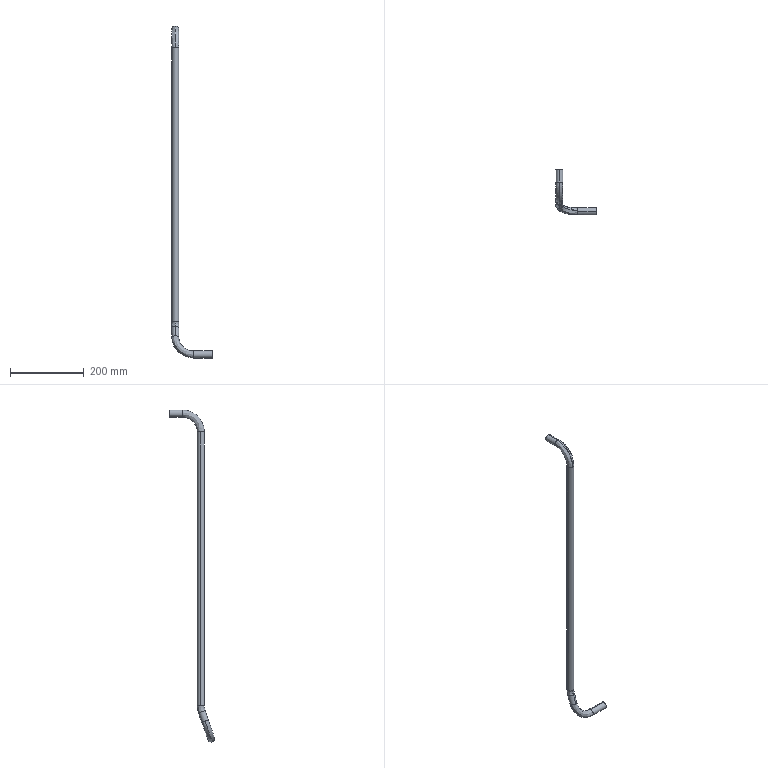Part | STEP file | copper tube 12_default_machined_ | 1 solid | 30 faces | box 109.5 x 122.5 x 899.3 mm | volume 84690 mm3 | cylinder 16 | spline 12 | plane 2 | commonest cylinder face diameters 16 x8 19 x8